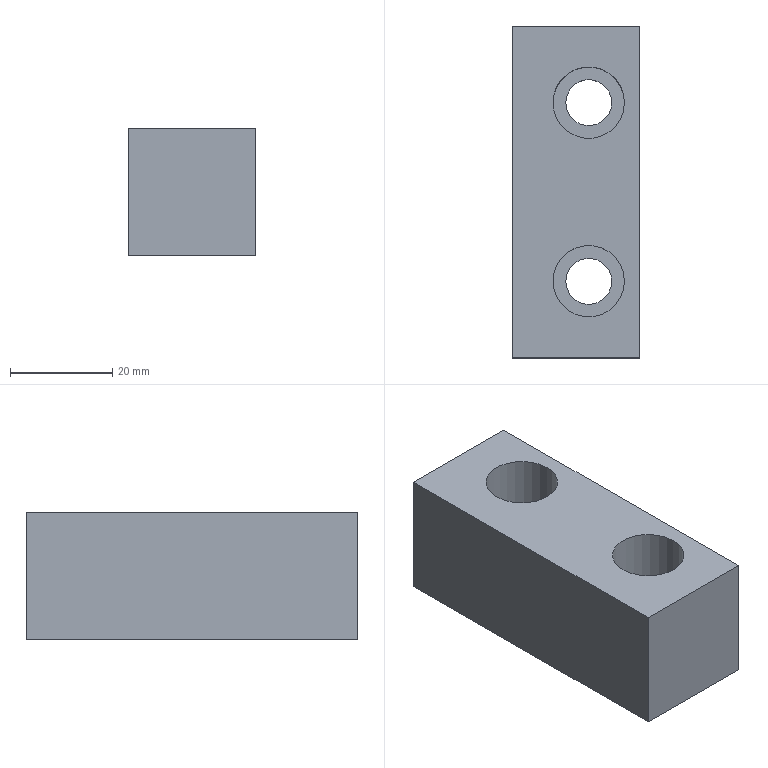Part | NX | features solid 2 | 1 solid | 12 faces | box 25 x 65 x 25 mm | volume 34735 mm3 | plane 8 | cylinder 4 | commonest cylinder face diameters 9 x2 14 x2
STEP:
#1=CARTESIAN_POINT('',(-1140.,-565.,-60.));
#2=VERTEX_POINT('',#1);
#3=CARTESIAN_POINT('',(-1115.,-565.,-60.));
#4=VERTEX_POINT('',#3);
#5=CARTESIAN_POINT('',(-1135.,-565.,-60.));
#6=DIRECTION('',(1.,0.,0.));
#7=VECTOR('',#6,1000.);
#8=LINE('',#5,#7);
#9=EDGE_CURVE('',#2,#4,#8,.T.);
#10=ORIENTED_EDGE('',*,*,#9,.F.);
#11=CARTESIAN_POINT('',(-1140.,-565.,-85.));
#12=VERTEX_POINT('',#11);
#13=CARTESIAN_POINT('',(-1140.,-565.,-35.));
#14=DIRECTION('',(0.,0.,-1.));
#15=VECTOR('',#14,1000.);
#16=LINE('',#13,#15);
#17=EDGE_CURVE('',#2,#12,#16,.T.);
#18=ORIENTED_EDGE('',*,*,#17,.T.);
#19=CARTESIAN_POINT('',(-1115.,-565.,-85.));
#20=VERTEX_POINT('',#19);
#21=CARTESIAN_POINT('',(149.393,-565.,-85.));
#22=DIRECTION('',(1.,0.,0.));
#23=VECTOR('',#22,1000.);
#24=LINE('',#21,#23);
#25=EDGE_CURVE('',#12,#20,#24,.T.);
#26=ORIENTED_EDGE('',*,*,#25,.T.);
#27=CARTESIAN_POINT('',(-1115.,-565.,-85.));
#28=DIRECTION('',(0.,0.,1.));
#29=VECTOR('',#28,1000.);
#30=LINE('',#27,#29);
#31=EDGE_CURVE('',#20,#4,#30,.T.);
#32=ORIENTED_EDGE('',*,*,#31,.T.);
#33=EDGE_LOOP('',(#10,#18,#26,#32));
#34=FACE_BOUND('',#33,.T.);
#35=CARTESIAN_POINT('',(149.393,-565.,-35.));
#36=DIRECTION('',(0.,-1.,0.));
#37=DIRECTION('',(0.,0.,-1.));
#38=AXIS2_PLACEMENT_3D('',#35,#36,#37);
#39=PLANE('',#38);
#40=ADVANCED_FACE('',(#34),#39,.T.);
#41=CARTESIAN_POINT('',(-1129.5,-515.,-85.));
#42=VERTEX_POINT('',#41);
#43=CARTESIAN_POINT('',(-1125.,-515.,-85.));
#44=DIRECTION('',(0.,0.,-1.));
#45=DIRECTION('',(-1.,0.,0.));
#46=AXIS2_PLACEMENT_3D('',#43,#44,#45);
#47=CIRCLE('',#46,4.5);
#48=EDGE_CURVE('',#42,#42,#47,.T.);
#49=ORIENTED_EDGE('',*,*,#48,.F.);
#50=EDGE_LOOP('',(#49));
#51=FACE_BOUND('',#50,.T.);
#52=CARTESIAN_POINT('',(-1129.5,-550.,-85.));
#53=VERTEX_POINT('',#52);
#54=CARTESIAN_POINT('',(-1125.,-550.,-85.));
#55=DIRECTION('',(0.,0.,-1.));
#56=DIRECTION('',(-1.,0.,0.));
#57=AXIS2_PLACEMENT_3D('',#54,#55,#56);
#58=CIRCLE('',#57,4.5);
#59=EDGE_CURVE('',#53,#53,#58,.T.);
#60=ORIENTED_EDGE('',*,*,#59,.F.);
#61=EDGE_LOOP('',(#60));
#62=FACE_BOUND('',#61,.T.);
#63=ORIENTED_EDGE('',*,*,#25,.F.);
#64=CARTESIAN_POINT('',(-1140.,-500.,-85.));
#65=VERTEX_POINT('',#64);
#66=CARTESIAN_POINT('',(-1140.,-450.,-85.));
#67=DIRECTION('',(0.,1.,0.));
#68=VECTOR('',#67,1000.);
#69=LINE('',#66,#68);
#70=EDGE_CURVE('',#12,#65,#69,.T.);
#71=ORIENTED_EDGE('',*,*,#70,.T.);
#72=CARTESIAN_POINT('',(-1115.,-500.,-85.));
#73=VERTEX_POINT('',#72);
#74=CARTESIAN_POINT('',(-1200.,-500.,-85.));
#75=DIRECTION('',(1.,0.,0.));
#76=VECTOR('',#75,1000.);
#77=LINE('',#74,#76);
#78=EDGE_CURVE('',#65,#73,#77,.T.);
#79=ORIENTED_EDGE('',*,*,#78,.T.);
#80=CARTESIAN_POINT('',(-1115.,-375.,-85.));
#81=DIRECTION('',(0.,1.,0.));
#82=VECTOR('',#81,1000.);
#83=LINE('',#80,#82);
#84=EDGE_CURVE('',#73,#20,#83,.F.);
#85=ORIENTED_EDGE('',*,*,#84,.T.);
#86=EDGE_LOOP('',(#63,#71,#79,#85));
#87=FACE_BOUND('',#86,.T.);
#88=CARTESIAN_POINT('',(-1185.,-450.,-85.));
#89=DIRECTION('',(0.,0.,-1.));
#90=DIRECTION('',(1.,0.,0.));
#91=AXIS2_PLACEMENT_3D('',#88,#89,#90);
#92=PLANE('',#91);
#93=ADVANCED_FACE('',(#51,#62,#87),#92,.T.);
#94=CARTESIAN_POINT('',(-1132.,-550.,-60.));
#95=VERTEX_POINT('',#94);
#96=CARTESIAN_POINT('',(-1125.,-550.,-60.));
#97=DIRECTION('',(0.,0.,-1.));
#98=DIRECTION('',(-1.,0.,0.));
#99=AXIS2_PLACEMENT_3D('',#96,#97,#98);
#100=CIRCLE('',#99,7.);
#101=EDGE_CURVE('',#95,#95,#100,.T.);
#102=ORIENTED_EDGE('',*,*,#101,.T.);
#103=EDGE_LOOP('',(#102));
#104=FACE_BOUND('',#103,.T.);
#105=CARTESIAN_POINT('',(-1132.,-515.,-60.));
#106=VERTEX_POINT('',#105);
#107=CARTESIAN_POINT('',(-1125.,-515.,-60.));
#108=DIRECTION('',(0.,0.,-1.));
#109=DIRECTION('',(-1.,0.,0.));
#110=AXIS2_PLACEMENT_3D('',#107,#108,#109);
#111=CIRCLE('',#110,7.);
#112=EDGE_CURVE('',#106,#106,#111,.T.);
#113=ORIENTED_EDGE('',*,*,#112,.T.);
#114=EDGE_LOOP('',(#113));
#115=FACE_BOUND('',#114,.T.);
#116=ORIENTED_EDGE('',*,*,#9,.T.);
#117=CARTESIAN_POINT('',(-1115.,-500.,-60.));
#118=VERTEX_POINT('',#117);
#119=CARTESIAN_POINT('',(-1115.,-375.,-60.));
#120=DIRECTION('',(0.,1.,0.));
#121=VECTOR('',#120,1000.);
#122=LINE('',#119,#121);
#123=EDGE_CURVE('',#118,#4,#122,.F.);
#124=ORIENTED_EDGE('',*,*,#123,.F.);
#125=CARTESIAN_POINT('',(-1140.,-500.,-60.));
#126=VERTEX_POINT('',#125);
#127=CARTESIAN_POINT('',(-1135.,-500.,-60.));
#128=DIRECTION('',(-1.,0.,0.));
#129=VECTOR('',#128,1000.);
#130=LINE('',#127,#129);
#131=EDGE_CURVE('',#126,#118,#130,.F.);
#132=ORIENTED_EDGE('',*,*,#131,.F.);
#133=CARTESIAN_POINT('',(-1140.,-375.,-60.));
#134=DIRECTION('',(0.,1.,0.));
#135=VECTOR('',#134,1000.);
#136=LINE('',#133,#135);
#137=EDGE_CURVE('',#126,#2,#136,.F.);
#138=ORIENTED_EDGE('',*,*,#137,.T.);
#139=EDGE_LOOP('',(#116,#124,#132,#138));
#140=FACE_BOUND('',#139,.T.);
#141=CARTESIAN_POINT('',(-1135.,-375.,-60.));
#142=DIRECTION('',(0.,0.,-1.));
#143=DIRECTION('',(0.,-1.,0.));
#144=AXIS2_PLACEMENT_3D('',#141,#142,#143);
#145=PLANE('',#144);
#146=ADVANCED_FACE('',(#104,#115,#140),#145,.F.);
#147=CARTESIAN_POINT('',(-1140.,-500.,-100.));
#148=DIRECTION('',(0.,0.,1.));
#149=VECTOR('',#148,1000.);
#150=LINE('',#147,#149);
#151=EDGE_CURVE('',#65,#126,#150,.T.);
#152=ORIENTED_EDGE('',*,*,#151,.T.);
#153=ORIENTED_EDGE('',*,*,#131,.T.);
#154=CARTESIAN_POINT('',(-1115.,-500.,-100.));
#155=DIRECTION('',(0.,0.,1.));
#156=VECTOR('',#155,1000.);
#157=LINE('',#154,#156);
#158=EDGE_CURVE('',#73,#118,#157,.T.);
#159=ORIENTED_EDGE('',*,*,#158,.F.);
#160=ORIENTED_EDGE('',*,*,#78,.F.);
#161=EDGE_LOOP('',(#152,#153,#159,#160));
#162=FACE_BOUND('',#161,.T.);
#163=CARTESIAN_POINT('',(-1200.,-500.,-100.));
#164=DIRECTION('',(0.,1.,0.));
#165=DIRECTION('',(1.,0.,0.));
#166=AXIS2_PLACEMENT_3D('',#163,#164,#165);
#167=PLANE('',#166);
#168=ADVANCED_FACE('',(#162),#167,.T.);
#169=ORIENTED_EDGE('',*,*,#123,.T.);
#170=ORIENTED_EDGE('',*,*,#31,.F.);
#171=ORIENTED_EDGE('',*,*,#84,.F.);
#172=ORIENTED_EDGE('',*,*,#158,.T.);
#173=EDGE_LOOP('',(#169,#170,#171,#172));
#174=FACE_BOUND('',#173,.T.);
#175=CARTESIAN_POINT('',(-1115.,-375.,-85.));
#176=DIRECTION('',(1.,0.,0.));
#177=DIRECTION('',(0.,0.,1.));
#178=AXIS2_PLACEMENT_3D('',#175,#176,#177);
#179=PLANE('',#178);
#180=ADVANCED_FACE('',(#174),#179,.T.);
#181=ORIENTED_EDGE('',*,*,#48,.T.);
#182=EDGE_LOOP('',(#181));
#183=FACE_BOUND('',#182,.T.);
#184=CARTESIAN_POINT('',(-1129.5,-515.,-75.));
#185=VERTEX_POINT('',#184);
#186=CARTESIAN_POINT('',(-1125.,-515.,-75.));
#187=DIRECTION('',(0.,0.,-1.));
#188=DIRECTION('',(-1.,0.,0.));
#189=AXIS2_PLACEMENT_3D('',#186,#187,#188);
#190=CIRCLE('',#189,4.5);
#191=EDGE_CURVE('',#185,#185,#190,.T.);
#192=ORIENTED_EDGE('',*,*,#191,.F.);
#193=EDGE_LOOP('',(#192));
#194=FACE_BOUND('',#193,.T.);
#195=CARTESIAN_POINT('',(-1125.,-515.,-110.));
#196=DIRECTION('',(0.,0.,-1.));
#197=DIRECTION('',(-1.,0.,0.));
#198=AXIS2_PLACEMENT_3D('',#195,#196,#197);
#199=CYLINDRICAL_SURFACE('',#198,4.5);
#200=ADVANCED_FACE('',(#183,#194),#199,.F.);
#201=ORIENTED_EDGE('',*,*,#191,.T.);
#202=EDGE_LOOP('',(#201));
#203=FACE_BOUND('',#202,.T.);
#204=CARTESIAN_POINT('',(-1132.,-515.,-75.));
#205=VERTEX_POINT('',#204);
#206=CARTESIAN_POINT('',(-1125.,-515.,-75.));
#207=DIRECTION('',(0.,0.,-1.));
#208=DIRECTION('',(-1.,0.,0.));
#209=AXIS2_PLACEMENT_3D('',#206,#207,#208);
#210=CIRCLE('',#209,7.);
#211=EDGE_CURVE('',#205,#205,#210,.T.);
#212=ORIENTED_EDGE('',*,*,#211,.F.);
#213=EDGE_LOOP('',(#212));
#214=FACE_BOUND('',#213,.T.);
#215=CARTESIAN_POINT('',(-1125.,-515.,-75.));
#216=DIRECTION('',(0.,0.,-1.));
#217=DIRECTION('',(-1.,0.,0.));
#218=AXIS2_PLACEMENT_3D('',#215,#216,#217);
#219=PLANE('',#218);
#220=ADVANCED_FACE('',(#203,#214),#219,.F.);
#221=ORIENTED_EDGE('',*,*,#211,.T.);
#222=EDGE_LOOP('',(#221));
#223=FACE_BOUND('',#222,.T.);
#224=ORIENTED_EDGE('',*,*,#112,.F.);
#225=EDGE_LOOP('',(#224));
#226=FACE_BOUND('',#225,.T.);
#227=CARTESIAN_POINT('',(-1125.,-515.,-60.));
#228=DIRECTION('',(0.,0.,-1.));
#229=DIRECTION('',(-1.,0.,0.));
#230=AXIS2_PLACEMENT_3D('',#227,#228,#229);
#231=CYLINDRICAL_SURFACE('',#230,7.);
#232=ADVANCED_FACE('',(#223,#226),#231,.F.);
#233=ORIENTED_EDGE('',*,*,#59,.T.);
#234=EDGE_LOOP('',(#233));
#235=FACE_BOUND('',#234,.T.);
#236=CARTESIAN_POINT('',(-1129.5,-550.,-75.));
#237=VERTEX_POINT('',#236);
#238=CARTESIAN_POINT('',(-1125.,-550.,-75.));
#239=DIRECTION('',(0.,0.,-1.));
#240=DIRECTION('',(-1.,0.,0.));
#241=AXIS2_PLACEMENT_3D('',#238,#239,#240);
#242=CIRCLE('',#241,4.5);
#243=EDGE_CURVE('',#237,#237,#242,.T.);
#244=ORIENTED_EDGE('',*,*,#243,.F.);
#245=EDGE_LOOP('',(#244));
#246=FACE_BOUND('',#245,.T.);
#247=CARTESIAN_POINT('',(-1125.,-550.,-110.));
#248=DIRECTION('',(0.,0.,-1.));
#249=DIRECTION('',(-1.,0.,0.));
#250=AXIS2_PLACEMENT_3D('',#247,#248,#249);
#251=CYLINDRICAL_SURFACE('',#250,4.5);
#252=ADVANCED_FACE('',(#235,#246),#251,.F.);
#253=ORIENTED_EDGE('',*,*,#243,.T.);
#254=EDGE_LOOP('',(#253));
#255=FACE_BOUND('',#254,.T.);
#256=CARTESIAN_POINT('',(-1132.,-550.,-75.));
#257=VERTEX_POINT('',#256);
#258=CARTESIAN_POINT('',(-1125.,-550.,-75.));
#259=DIRECTION('',(0.,0.,-1.));
#260=DIRECTION('',(-1.,0.,0.));
#261=AXIS2_PLACEMENT_3D('',#258,#259,#260);
#262=CIRCLE('',#261,7.);
#263=EDGE_CURVE('',#257,#257,#262,.T.);
#264=ORIENTED_EDGE('',*,*,#263,.F.);
#265=EDGE_LOOP('',(#264));
#266=FACE_BOUND('',#265,.T.);
#267=CARTESIAN_POINT('',(-1125.,-550.,-75.));
#268=DIRECTION('',(0.,0.,-1.));
#269=DIRECTION('',(-1.,0.,0.));
#270=AXIS2_PLACEMENT_3D('',#267,#268,#269);
#271=PLANE('',#270);
#272=ADVANCED_FACE('',(#255,#266),#271,.F.);
#273=ORIENTED_EDGE('',*,*,#263,.T.);
#274=EDGE_LOOP('',(#273));
#275=FACE_BOUND('',#274,.T.);
#276=ORIENTED_EDGE('',*,*,#101,.F.);
#277=EDGE_LOOP('',(#276));
#278=FACE_BOUND('',#277,.T.);
#279=CARTESIAN_POINT('',(-1125.,-550.,-60.));
#280=DIRECTION('',(0.,0.,-1.));
#281=DIRECTION('',(-1.,0.,0.));
#282=AXIS2_PLACEMENT_3D('',#279,#280,#281);
#283=CYLINDRICAL_SURFACE('',#282,7.);
#284=ADVANCED_FACE('',(#275,#278),#283,.F.);
#285=ORIENTED_EDGE('',*,*,#17,.F.);
#286=ORIENTED_EDGE('',*,*,#137,.F.);
#287=ORIENTED_EDGE('',*,*,#151,.F.);
#288=ORIENTED_EDGE('',*,*,#70,.F.);
#289=EDGE_LOOP('',(#285,#286,#287,#288));
#290=FACE_BOUND('',#289,.T.);
#291=CARTESIAN_POINT('',(-1140.,1085.,-60.));
#292=DIRECTION('',(-1.,0.,0.));
#293=DIRECTION('',(0.,0.,1.));
#294=AXIS2_PLACEMENT_3D('',#291,#292,#293);
#295=PLANE('',#294);
#296=ADVANCED_FACE('',(#290),#295,.T.);
#297=CLOSED_SHELL('',(#40,#93,#146,#168,#180,#200,#220,#232,#252,#272,#284,#296));
#298=MANIFOLD_SOLID_BREP('',#297);
#299=(LENGTH_UNIT()NAMED_UNIT(*)SI_UNIT(.MILLI.,.METRE.));
#300=UNCERTAINTY_MEASURE_WITH_UNIT(LENGTH_MEASURE(0.00001),#299,'','');
#301=(NAMED_UNIT(*)PLANE_ANGLE_UNIT()SI_UNIT($,.RADIAN.));
#302=(NAMED_UNIT(*)SI_UNIT($,.STERADIAN.)SOLID_ANGLE_UNIT());
#303=(GEOMETRIC_REPRESENTATION_CONTEXT(3)GLOBAL_UNCERTAINTY_ASSIGNED_CONTEXT((#300))GLOBAL_UNIT_ASSIGNED_CONTEXT((#299,#301,#302))REPRESENTATION_CONTEXT('',''));
#304=ADVANCED_BREP_SHAPE_REPRESENTATION('',(#298),#303);